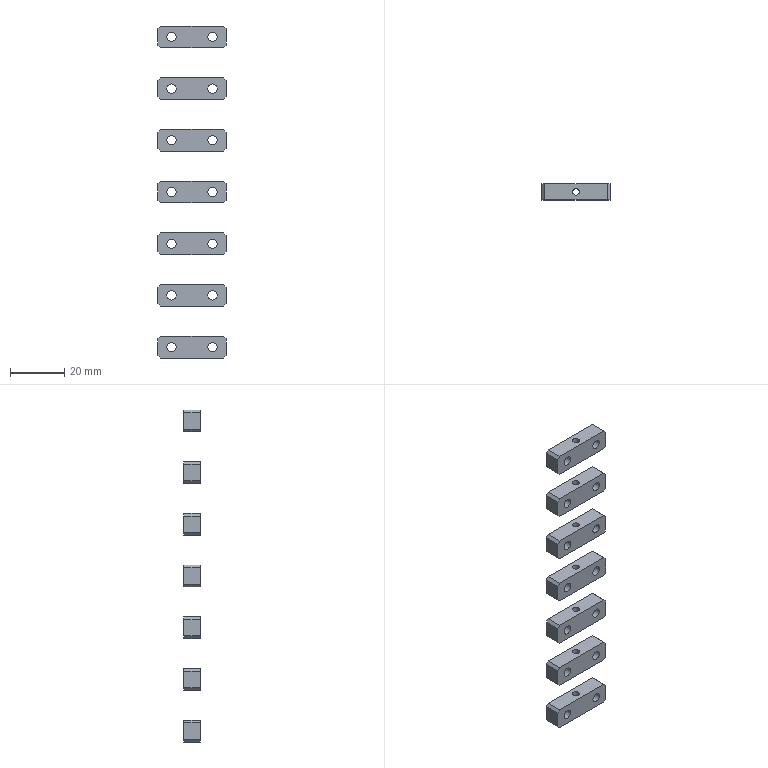Part | 7 solids | 119 faces | box 25 x 6 x 122 mm | volume 6365 mm3 | plane 84 | cylinder 35 | commonest cylinder face diameters 3.4 x14 6 x14 2.5 x7